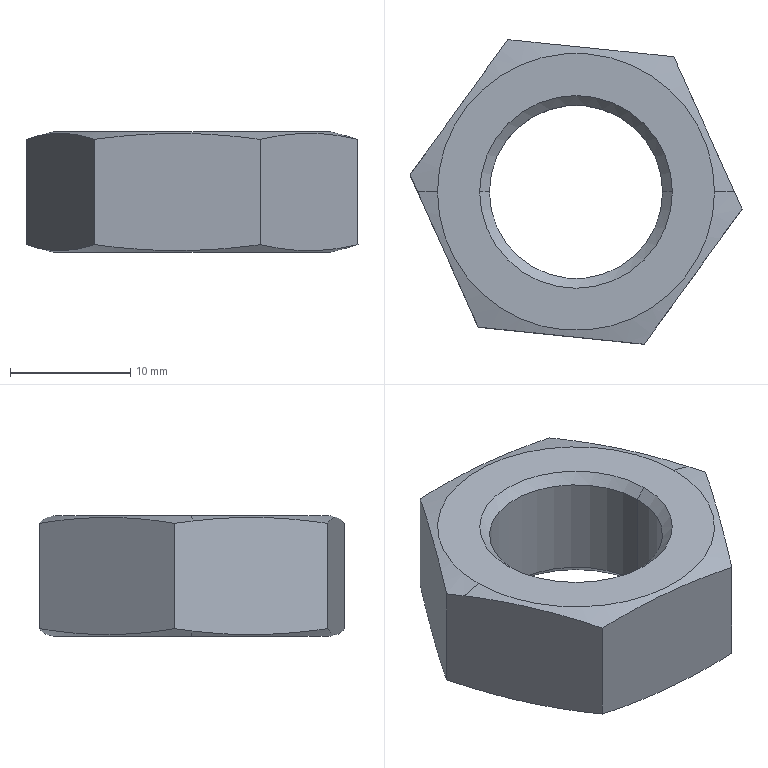Part | SolidWorks | features BaseBody 1 | 1 solid | 18 faces | box 27.567 x 25.293 x 10 mm | volume 3303 mm3 | cone 8 | plane 8 | cylinder 2 | commonest cylinder face diameters 14.376 x2
STEP:
#1=CARTESIAN_POINT('',(223.5,0.,-23.475));
#2=VERTEX_POINT('',#1);
#3=CARTESIAN_POINT('',(246.5,0.,-23.475));
#4=VERTEX_POINT('',#3);
#5=CARTESIAN_POINT('',(235.,0.,-23.475));
#6=DIRECTION('',(0.,0.,-1.));
#7=DIRECTION('',(1.,0.,0.));
#8=AXIS2_PLACEMENT_3D('',#5,#6,#7);
#9=CIRCLE('',#8,11.5);
#10=EDGE_CURVE('',#2,#4,#9,.T.);
#11=ORIENTED_EDGE('',*,*,#10,.F.);
#12=CARTESIAN_POINT('',(221.852,0.,-23.033));
#13=VERTEX_POINT('',#12);
#14=CARTESIAN_POINT('',(221.129,0.,-22.839));
#15=DIRECTION('',(-0.9659,0.,0.2588));
#16=VECTOR('',#15,1000.);
#17=LINE('',#14,#16);
#18=EDGE_CURVE('',#2,#13,#17,.T.);
#19=ORIENTED_EDGE('',*,*,#18,.T.);
#20=CARTESIAN_POINT('',(221.216,1.419,-22.843));
#21=VERTEX_POINT('',#20);
#22=CARTESIAN_POINT('',(221.852,0.,-23.033));
#23=CARTESIAN_POINT('',(221.64,0.4732,-22.976));
#24=CARTESIAN_POINT('',(221.428,0.9463,-22.913));
#25=CARTESIAN_POINT('',(221.216,1.419,-22.843));
#26=B_SPLINE_CURVE_WITH_KNOTS('',3,(#22,#23,#24,#25),.UNSPECIFIED.,.F.,.F.,(4,4),(0.0123,0.01386),.UNSPECIFIED.);
#27=EDGE_CURVE('',#13,#21,#26,.T.);
#28=ORIENTED_EDGE('',*,*,#27,.T.);
#29=CARTESIAN_POINT('',(229.338,12.647,-22.843));
#30=VERTEX_POINT('',#29);
#31=CARTESIAN_POINT('',(221.216,1.419,-22.843));
#32=CARTESIAN_POINT('',(221.893,2.355,-22.998));
#33=CARTESIAN_POINT('',(222.57,3.291,-23.124));
#34=CARTESIAN_POINT('',(223.924,5.162,-23.295));
#35=CARTESIAN_POINT('',(225.277,7.033,-23.386));
#36=CARTESIAN_POINT('',(226.631,8.904,-23.295));
#37=CARTESIAN_POINT('',(227.984,10.775,-23.124));
#38=CARTESIAN_POINT('',(228.661,11.711,-22.998));
#39=CARTESIAN_POINT('',(229.338,12.647,-22.843));
#40=B_SPLINE_CURVE_WITH_KNOTS('',3,(#31,#32,#33,#34,#35,#36,#37,#38,#39),.UNSPECIFIED.,.F.,.F.,(4,2,1,2,4),(0.,0.003464,0.006928,0.01039,0.01386),.UNSPECIFIED.);
#41=EDGE_CURVE('',#21,#30,#40,.T.);
#42=ORIENTED_EDGE('',*,*,#41,.T.);
#43=CARTESIAN_POINT('',(243.121,11.227,-22.843));
#44=VERTEX_POINT('',#43);
#45=CARTESIAN_POINT('',(229.338,12.647,-22.843));
#46=CARTESIAN_POINT('',(230.481,12.529,-22.997));
#47=CARTESIAN_POINT('',(231.627,12.411,-23.123));
#48=CARTESIAN_POINT('',(233.924,12.174,-23.295));
#49=CARTESIAN_POINT('',(235.075,12.056,-23.341));
#50=CARTESIAN_POINT('',(237.384,11.818,-23.341));
#51=CARTESIAN_POINT('',(238.535,11.699,-23.295));
#52=CARTESIAN_POINT('',(240.832,11.463,-23.123));
#53=CARTESIAN_POINT('',(241.978,11.345,-22.997));
#54=CARTESIAN_POINT('',(243.121,11.227,-22.843));
#55=B_SPLINE_CURVE_WITH_KNOTS('',3,(#45,#46,#47,#48,#49,#50,#51,#52,#53,#54),.UNSPECIFIED.,.F.,.F.,(4,2,2,2,4),(-0.006946,-0.003473,0.,0.003473,0.006946),.UNSPECIFIED.);
#56=EDGE_CURVE('',#30,#44,#55,.T.);
#57=ORIENTED_EDGE('',*,*,#56,.T.);
#58=CARTESIAN_POINT('',(248.148,0.,-23.033));
#59=VERTEX_POINT('',#58);
#60=CARTESIAN_POINT('',(243.121,11.227,-22.843));
#61=CARTESIAN_POINT('',(243.959,9.356,-23.118));
#62=CARTESIAN_POINT('',(244.797,7.485,-23.298));
#63=CARTESIAN_POINT('',(246.053,4.678,-23.352));
#64=CARTESIAN_POINT('',(246.472,3.742,-23.334));
#65=CARTESIAN_POINT('',(247.31,1.871,-23.231));
#66=CARTESIAN_POINT('',(247.729,0.9356,-23.145));
#67=CARTESIAN_POINT('',(248.148,0.,-23.033));
#68=B_SPLINE_CURVE_WITH_KNOTS('',3,(#60,#61,#62,#63,#64,#65,#66,#67),.UNSPECIFIED.,.F.,.F.,(4,2,2,4),(0.,0.006151,0.009226,0.0123),.UNSPECIFIED.);
#69=EDGE_CURVE('',#44,#59,#68,.T.);
#70=ORIENTED_EDGE('',*,*,#69,.T.);
#71=CARTESIAN_POINT('',(248.871,0.,-22.839));
#72=DIRECTION('',(0.9659,0.,0.2588));
#73=VECTOR('',#72,1000.);
#74=LINE('',#71,#73);
#75=EDGE_CURVE('',#4,#59,#74,.T.);
#76=ORIENTED_EDGE('',*,*,#75,.F.);
#77=EDGE_LOOP('',(#11,#19,#28,#42,#57,#70,#76));
#78=FACE_OUTER_BOUND('',#77,.T.);
#79=CARTESIAN_POINT('',(235.,0.,-22.839));
#80=DIRECTION('',(0.,0.,1.));
#81=DIRECTION('',(1.,0.,0.));
#82=AXIS2_PLACEMENT_3D('',#79,#80,#81);
#83=CONICAL_SURFACE('',#82,13.871,1.309);
#84=ADVANCED_FACE('',(#78),#83,.T.);
#85=CARTESIAN_POINT('',(242.188,0.,-22.663));
#86=VERTEX_POINT('',#85);
#87=CARTESIAN_POINT('',(227.812,0.,-22.663));
#88=VERTEX_POINT('',#87);
#89=CARTESIAN_POINT('',(235.,0.,-22.663));
#90=DIRECTION('',(0.,0.,-1.));
#91=DIRECTION('',(0.1024,0.9947,0.));
#92=AXIS2_PLACEMENT_3D('',#89,#90,#91);
#93=CIRCLE('',#92,7.188);
#94=EDGE_CURVE('',#86,#88,#93,.T.);
#95=ORIENTED_EDGE('',*,*,#94,.F.);
#96=CARTESIAN_POINT('',(243.,0.,-23.475));
#97=VERTEX_POINT('',#96);
#98=CARTESIAN_POINT('',(243.,0.,-23.475));
#99=DIRECTION('',(0.7071,0.,-0.7071));
#100=VECTOR('',#99,1000.);
#101=LINE('',#98,#100);
#102=EDGE_CURVE('',#86,#97,#101,.T.);
#103=ORIENTED_EDGE('',*,*,#102,.T.);
#104=CARTESIAN_POINT('',(227.,0.,-23.475));
#105=VERTEX_POINT('',#104);
#106=CARTESIAN_POINT('',(235.,0.,-23.475));
#107=DIRECTION('',(0.,0.,1.));
#108=DIRECTION('',(-1.,0.,0.));
#109=AXIS2_PLACEMENT_3D('',#106,#107,#108);
#110=CIRCLE('',#109,8.);
#111=EDGE_CURVE('',#105,#97,#110,.T.);
#112=ORIENTED_EDGE('',*,*,#111,.F.);
#113=CARTESIAN_POINT('',(227.,0.,-23.475));
#114=DIRECTION('',(-0.7071,0.,-0.7071));
#115=VECTOR('',#114,1000.);
#116=LINE('',#113,#115);
#117=EDGE_CURVE('',#88,#105,#116,.T.);
#118=ORIENTED_EDGE('',*,*,#117,.F.);
#119=EDGE_LOOP('',(#95,#103,#112,#118));
#120=FACE_OUTER_BOUND('',#119,.T.);
#121=CARTESIAN_POINT('',(235.,0.,-23.475));
#122=DIRECTION('',(0.,0.,-1.));
#123=DIRECTION('',(-1.,0.,0.));
#124=AXIS2_PLACEMENT_3D('',#121,#122,#123);
#125=CONICAL_SURFACE('',#124,8.,0.7854);
#126=ADVANCED_FACE('',(#120),#125,.F.);
#127=CARTESIAN_POINT('',(242.188,0.,-14.287));
#128=VERTEX_POINT('',#127);
#129=CARTESIAN_POINT('',(227.812,0.,-14.287));
#130=VERTEX_POINT('',#129);
#131=CARTESIAN_POINT('',(235.,0.,-14.287));
#132=DIRECTION('',(0.,0.,-1.));
#133=DIRECTION('',(-1.,0.,0.));
#134=AXIS2_PLACEMENT_3D('',#131,#132,#133);
#135=CIRCLE('',#134,7.188);
#136=EDGE_CURVE('',#128,#130,#135,.T.);
#137=ORIENTED_EDGE('',*,*,#136,.F.);
#138=CARTESIAN_POINT('',(242.188,0.,-18.475));
#139=DIRECTION('',(0.,0.,-1.));
#140=VECTOR('',#139,1000.);
#141=LINE('',#138,#140);
#142=EDGE_CURVE('',#128,#86,#141,.T.);
#143=ORIENTED_EDGE('',*,*,#142,.T.);
#144=ORIENTED_EDGE('',*,*,#94,.T.);
#145=CARTESIAN_POINT('',(227.812,0.,-18.475));
#146=DIRECTION('',(0.,0.,-1.));
#147=VECTOR('',#146,1000.);
#148=LINE('',#145,#147);
#149=EDGE_CURVE('',#130,#88,#148,.T.);
#150=ORIENTED_EDGE('',*,*,#149,.F.);
#151=EDGE_LOOP('',(#137,#143,#144,#150));
#152=FACE_OUTER_BOUND('',#151,.T.);
#153=CARTESIAN_POINT('',(235.,0.,-18.475));
#154=DIRECTION('',(0.,0.,-1.));
#155=DIRECTION('',(-1.,0.,0.));
#156=AXIS2_PLACEMENT_3D('',#153,#154,#155);
#157=CYLINDRICAL_SURFACE('',#156,7.188);
#158=ADVANCED_FACE('',(#152),#157,.F.);
#159=CARTESIAN_POINT('',(223.5,0.,-13.475));
#160=VERTEX_POINT('',#159);
#161=CARTESIAN_POINT('',(246.5,0.,-13.475));
#162=VERTEX_POINT('',#161);
#163=CARTESIAN_POINT('',(235.,0.,-13.475));
#164=DIRECTION('',(0.,0.,-1.));
#165=DIRECTION('',(-1.,0.,0.));
#166=AXIS2_PLACEMENT_3D('',#163,#164,#165);
#167=CIRCLE('',#166,11.5);
#168=EDGE_CURVE('',#160,#162,#167,.T.);
#169=ORIENTED_EDGE('',*,*,#168,.T.);
#170=CARTESIAN_POINT('',(248.148,0.,-13.916));
#171=VERTEX_POINT('',#170);
#172=CARTESIAN_POINT('',(248.871,0.,-14.11));
#173=DIRECTION('',(0.9659,0.,-0.2588));
#174=VECTOR('',#173,1000.);
#175=LINE('',#172,#174);
#176=EDGE_CURVE('',#162,#171,#175,.T.);
#177=ORIENTED_EDGE('',*,*,#176,.T.);
#178=CARTESIAN_POINT('',(243.121,11.227,-14.106));
#179=VERTEX_POINT('',#178);
#180=CARTESIAN_POINT('',(248.148,0.,-13.916));
#181=CARTESIAN_POINT('',(247.729,0.9356,-13.804));
#182=CARTESIAN_POINT('',(247.31,1.871,-13.719));
#183=CARTESIAN_POINT('',(246.472,3.742,-13.615));
#184=CARTESIAN_POINT('',(246.053,4.678,-13.598));
#185=CARTESIAN_POINT('',(244.797,7.485,-13.651));
#186=CARTESIAN_POINT('',(243.959,9.356,-13.831));
#187=CARTESIAN_POINT('',(243.121,11.227,-14.106));
#188=B_SPLINE_CURVE_WITH_KNOTS('',3,(#180,#181,#182,#183,#184,#185,#186,#187),.UNSPECIFIED.,.F.,.F.,(4,2,2,4),(0.001555,0.004631,0.007706,0.01386),.UNSPECIFIED.);
#189=EDGE_CURVE('',#171,#179,#188,.T.);
#190=ORIENTED_EDGE('',*,*,#189,.T.);
#191=CARTESIAN_POINT('',(229.338,12.647,-14.106));
#192=VERTEX_POINT('',#191);
#193=CARTESIAN_POINT('',(243.121,11.227,-14.106));
#194=CARTESIAN_POINT('',(241.978,11.345,-13.952));
#195=CARTESIAN_POINT('',(240.832,11.463,-13.826));
#196=CARTESIAN_POINT('',(238.535,11.699,-13.655));
#197=CARTESIAN_POINT('',(237.384,11.818,-13.609));
#198=CARTESIAN_POINT('',(235.075,12.056,-13.609));
#199=CARTESIAN_POINT('',(233.924,12.174,-13.655));
#200=CARTESIAN_POINT('',(231.627,12.411,-13.826));
#201=CARTESIAN_POINT('',(230.481,12.529,-13.952));
#202=CARTESIAN_POINT('',(229.338,12.647,-14.106));
#203=B_SPLINE_CURVE_WITH_KNOTS('',3,(#193,#194,#195,#196,#197,#198,#199,#200,#201,#202),.UNSPECIFIED.,.F.,.F.,(4,2,2,2,4),(-0.006946,-0.003473,0.,0.003473,0.006946),.UNSPECIFIED.);
#204=EDGE_CURVE('',#179,#192,#203,.T.);
#205=ORIENTED_EDGE('',*,*,#204,.T.);
#206=CARTESIAN_POINT('',(221.216,1.419,-14.106));
#207=VERTEX_POINT('',#206);
#208=CARTESIAN_POINT('',(229.338,12.647,-14.106));
#209=CARTESIAN_POINT('',(228.661,11.711,-13.951));
#210=CARTESIAN_POINT('',(227.984,10.775,-13.826));
#211=CARTESIAN_POINT('',(226.631,8.904,-13.654));
#212=CARTESIAN_POINT('',(225.277,7.033,-13.563));
#213=CARTESIAN_POINT('',(223.924,5.162,-13.654));
#214=CARTESIAN_POINT('',(222.57,3.291,-13.826));
#215=CARTESIAN_POINT('',(221.893,2.355,-13.951));
#216=CARTESIAN_POINT('',(221.216,1.419,-14.106));
#217=B_SPLINE_CURVE_WITH_KNOTS('',3,(#208,#209,#210,#211,#212,#213,#214,#215,#216),.UNSPECIFIED.,.F.,.F.,(4,2,1,2,4),(0.,0.003464,0.006928,0.01039,0.01386),.UNSPECIFIED.);
#218=EDGE_CURVE('',#192,#207,#217,.T.);
#219=ORIENTED_EDGE('',*,*,#218,.T.);
#220=CARTESIAN_POINT('',(221.852,0.,-13.916));
#221=VERTEX_POINT('',#220);
#222=CARTESIAN_POINT('',(221.216,1.419,-14.106));
#223=CARTESIAN_POINT('',(221.428,0.9463,-14.037));
#224=CARTESIAN_POINT('',(221.64,0.4732,-13.973));
#225=CARTESIAN_POINT('',(221.852,0.,-13.916));
#226=B_SPLINE_CURVE_WITH_KNOTS('',3,(#222,#223,#224,#225),.UNSPECIFIED.,.F.,.F.,(4,4),(0.,0.001555),.UNSPECIFIED.);
#227=EDGE_CURVE('',#207,#221,#226,.T.);
#228=ORIENTED_EDGE('',*,*,#227,.T.);
#229=CARTESIAN_POINT('',(221.129,0.,-14.11));
#230=DIRECTION('',(-0.9659,0.,-0.2588));
#231=VECTOR('',#230,1000.);
#232=LINE('',#229,#231);
#233=EDGE_CURVE('',#160,#221,#232,.T.);
#234=ORIENTED_EDGE('',*,*,#233,.F.);
#235=EDGE_LOOP('',(#169,#177,#190,#205,#219,#228,#234));
#236=FACE_OUTER_BOUND('',#235,.T.);
#237=CARTESIAN_POINT('',(235.,0.,-14.11));
#238=DIRECTION('',(0.,0.,-1.));
#239=DIRECTION('',(-1.,0.,0.));
#240=AXIS2_PLACEMENT_3D('',#237,#238,#239);
#241=CONICAL_SURFACE('',#240,13.871,1.309);
#242=ADVANCED_FACE('',(#236),#241,.T.);
#243=ORIENTED_EDGE('',*,*,#136,.T.);
#244=CARTESIAN_POINT('',(227.,0.,-13.475));
#245=VERTEX_POINT('',#244);
#246=CARTESIAN_POINT('',(227.,0.,-13.475));
#247=DIRECTION('',(-0.7071,0.,0.7071));
#248=VECTOR('',#247,1000.);
#249=LINE('',#246,#248);
#250=EDGE_CURVE('',#130,#245,#249,.T.);
#251=ORIENTED_EDGE('',*,*,#250,.T.);
#252=CARTESIAN_POINT('',(243.,0.,-13.475));
#253=VERTEX_POINT('',#252);
#254=CARTESIAN_POINT('',(235.,0.,-13.475));
#255=DIRECTION('',(0.,0.,-1.));
#256=DIRECTION('',(1.,0.,0.));
#257=AXIS2_PLACEMENT_3D('',#254,#255,#256);
#258=CIRCLE('',#257,8.);
#259=EDGE_CURVE('',#253,#245,#258,.T.);
#260=ORIENTED_EDGE('',*,*,#259,.F.);
#261=CARTESIAN_POINT('',(243.,0.,-13.475));
#262=DIRECTION('',(0.7071,0.,0.7071));
#263=VECTOR('',#262,1000.);
#264=LINE('',#261,#263);
#265=EDGE_CURVE('',#128,#253,#264,.T.);
#266=ORIENTED_EDGE('',*,*,#265,.F.);
#267=EDGE_LOOP('',(#243,#251,#260,#266));
#268=FACE_OUTER_BOUND('',#267,.T.);
#269=CARTESIAN_POINT('',(235.,0.,-13.475));
#270=DIRECTION('',(0.,0.,1.));
#271=DIRECTION('',(1.,0.,0.));
#272=AXIS2_PLACEMENT_3D('',#269,#270,#271);
#273=CONICAL_SURFACE('',#272,8.,0.7854);
#274=ADVANCED_FACE('',(#268),#273,.F.);
#275=CARTESIAN_POINT('',(235.,0.,-23.475));
#276=DIRECTION('',(0.,0.,-1.));
#277=DIRECTION('',(1.,0.,0.));
#278=AXIS2_PLACEMENT_3D('',#275,#276,#277);
#279=CIRCLE('',#278,11.5);
#280=EDGE_CURVE('',#4,#2,#279,.T.);
#281=ORIENTED_EDGE('',*,*,#280,.T.);
#282=ORIENTED_EDGE('',*,*,#10,.T.);
#283=EDGE_LOOP('',(#281,#282));
#284=FACE_OUTER_BOUND('',#283,.T.);
#285=ORIENTED_EDGE('',*,*,#111,.T.);
#286=CARTESIAN_POINT('',(235.,0.,-23.475));
#287=DIRECTION('',(0.,0.,1.));
#288=DIRECTION('',(-1.,0.,0.));
#289=AXIS2_PLACEMENT_3D('',#286,#287,#288);
#290=CIRCLE('',#289,8.);
#291=EDGE_CURVE('',#97,#105,#290,.T.);
#292=ORIENTED_EDGE('',*,*,#291,.T.);
#293=EDGE_LOOP('',(#285,#292));
#294=FACE_BOUND('',#293,.T.);
#295=CARTESIAN_POINT('',(225.301,0.9988,-23.475));
#296=DIRECTION('',(0.,0.,-1.));
#297=DIRECTION('',(-1.,0.,0.));
#298=AXIS2_PLACEMENT_3D('',#295,#296,#297);
#299=PLANE('',#298);
#300=ADVANCED_FACE('',(#284,#294),#299,.T.);
#301=ORIENTED_EDGE('',*,*,#18,.F.);
#302=ORIENTED_EDGE('',*,*,#280,.F.);
#303=ORIENTED_EDGE('',*,*,#75,.T.);
#304=CARTESIAN_POINT('',(248.784,-1.419,-22.843));
#305=VERTEX_POINT('',#304);
#306=CARTESIAN_POINT('',(248.148,0.,-23.033));
#307=CARTESIAN_POINT('',(248.36,-0.4732,-22.976));
#308=CARTESIAN_POINT('',(248.572,-0.9463,-22.913));
#309=CARTESIAN_POINT('',(248.784,-1.419,-22.843));
#310=B_SPLINE_CURVE_WITH_KNOTS('',3,(#306,#307,#308,#309),.UNSPECIFIED.,.F.,.F.,(4,4),(0.0123,0.01386),.UNSPECIFIED.);
#311=EDGE_CURVE('',#59,#305,#310,.T.);
#312=ORIENTED_EDGE('',*,*,#311,.T.);
#313=CARTESIAN_POINT('',(240.662,-12.647,-22.843));
#314=VERTEX_POINT('',#313);
#315=CARTESIAN_POINT('',(248.784,-1.419,-22.843));
#316=CARTESIAN_POINT('',(248.107,-2.355,-22.998));
#317=CARTESIAN_POINT('',(247.43,-3.291,-23.124));
#318=CARTESIAN_POINT('',(246.076,-5.162,-23.295));
#319=CARTESIAN_POINT('',(244.723,-7.033,-23.386));
#320=CARTESIAN_POINT('',(243.369,-8.904,-23.295));
#321=CARTESIAN_POINT('',(242.016,-10.775,-23.124));
#322=CARTESIAN_POINT('',(241.339,-11.711,-22.998));
#323=CARTESIAN_POINT('',(240.662,-12.647,-22.843));
#324=B_SPLINE_CURVE_WITH_KNOTS('',3,(#315,#316,#317,#318,#319,#320,#321,#322,#323),.UNSPECIFIED.,.F.,.F.,(4,2,1,2,4),(0.,0.003464,0.006928,0.01039,0.01386),.UNSPECIFIED.);
#325=EDGE_CURVE('',#305,#314,#324,.T.);
#326=ORIENTED_EDGE('',*,*,#325,.T.);
#327=CARTESIAN_POINT('',(226.879,-11.227,-22.843));
#328=VERTEX_POINT('',#327);
#329=CARTESIAN_POINT('',(240.662,-12.647,-22.843));
#330=CARTESIAN_POINT('',(239.519,-12.529,-22.997));
#331=CARTESIAN_POINT('',(238.373,-12.411,-23.123));
#332=CARTESIAN_POINT('',(236.076,-12.174,-23.295));
#333=CARTESIAN_POINT('',(234.925,-12.056,-23.341));
#334=CARTESIAN_POINT('',(232.616,-11.818,-23.341));
#335=CARTESIAN_POINT('',(231.465,-11.699,-23.295));
#336=CARTESIAN_POINT('',(229.168,-11.463,-23.123));
#337=CARTESIAN_POINT('',(228.022,-11.345,-22.997));
#338=CARTESIAN_POINT('',(226.879,-11.227,-22.843));
#339=B_SPLINE_CURVE_WITH_KNOTS('',3,(#329,#330,#331,#332,#333,#334,#335,#336,#337,#338),.UNSPECIFIED.,.F.,.F.,(4,2,2,2,4),(-0.006946,-0.003473,0.,0.003473,0.006946),.UNSPECIFIED.);
#340=EDGE_CURVE('',#314,#328,#339,.T.);
#341=ORIENTED_EDGE('',*,*,#340,.T.);
#342=CARTESIAN_POINT('',(226.879,-11.227,-22.843));
#343=CARTESIAN_POINT('',(226.041,-9.356,-23.118));
#344=CARTESIAN_POINT('',(225.203,-7.485,-23.298));
#345=CARTESIAN_POINT('',(223.947,-4.678,-23.352));
#346=CARTESIAN_POINT('',(223.528,-3.742,-23.334));
#347=CARTESIAN_POINT('',(222.69,-1.871,-23.231));
#348=CARTESIAN_POINT('',(222.271,-0.9356,-23.145));
#349=CARTESIAN_POINT('',(221.852,0.,-23.033));
#350=B_SPLINE_CURVE_WITH_KNOTS('',3,(#342,#343,#344,#345,#346,#347,#348,#349),.UNSPECIFIED.,.F.,.F.,(4,2,2,4),(0.,0.006151,0.009226,0.0123),.UNSPECIFIED.);
#351=EDGE_CURVE('',#328,#13,#350,.T.);
#352=ORIENTED_EDGE('',*,*,#351,.T.);
#353=EDGE_LOOP('',(#301,#302,#303,#312,#326,#341,#352));
#354=FACE_OUTER_BOUND('',#353,.T.);
#355=CARTESIAN_POINT('',(235.,0.,-22.839));
#356=DIRECTION('',(0.,0.,1.));
#357=DIRECTION('',(1.,0.,0.));
#358=AXIS2_PLACEMENT_3D('',#355,#356,#357);
#359=CONICAL_SURFACE('',#358,13.871,1.309);
#360=ADVANCED_FACE('',(#354),#359,.T.);
#361=ORIENTED_EDGE('',*,*,#102,.F.);
#362=CARTESIAN_POINT('',(235.,0.,-22.663));
#363=DIRECTION('',(0.,0.,-1.));
#364=DIRECTION('',(0.1024,0.9947,0.));
#365=AXIS2_PLACEMENT_3D('',#362,#363,#364);
#366=CIRCLE('',#365,7.188);
#367=EDGE_CURVE('',#88,#86,#366,.T.);
#368=ORIENTED_EDGE('',*,*,#367,.F.);
#369=ORIENTED_EDGE('',*,*,#117,.T.);
#370=ORIENTED_EDGE('',*,*,#291,.F.);
#371=EDGE_LOOP('',(#361,#368,#369,#370));
#372=FACE_OUTER_BOUND('',#371,.T.);
#373=CARTESIAN_POINT('',(235.,0.,-23.475));
#374=DIRECTION('',(0.,0.,-1.));
#375=DIRECTION('',(-1.,0.,0.));
#376=AXIS2_PLACEMENT_3D('',#373,#374,#375);
#377=CONICAL_SURFACE('',#376,8.,0.7854);
#378=ADVANCED_FACE('',(#372),#377,.F.);
#379=CARTESIAN_POINT('',(248.784,-1.419,-14.106));
#380=VERTEX_POINT('',#379);
#381=CARTESIAN_POINT('',(248.784,-1.419,-14.106));
#382=CARTESIAN_POINT('',(248.572,-0.9463,-14.037));
#383=CARTESIAN_POINT('',(248.36,-0.4732,-13.973));
#384=CARTESIAN_POINT('',(248.148,0.,-13.916));
#385=B_SPLINE_CURVE_WITH_KNOTS('',3,(#381,#382,#383,#384),.UNSPECIFIED.,.F.,.F.,(4,4),(0.,0.001555),.UNSPECIFIED.);
#386=EDGE_CURVE('',#380,#171,#385,.T.);
#387=ORIENTED_EDGE('',*,*,#386,.F.);
#388=CARTESIAN_POINT('',(248.784,-1.419,-23.475));
#389=DIRECTION('',(0.,0.,1.));
#390=VECTOR('',#389,1000.);
#391=LINE('',#388,#390);
#392=EDGE_CURVE('',#305,#380,#391,.T.);
#393=ORIENTED_EDGE('',*,*,#392,.F.);
#394=ORIENTED_EDGE('',*,*,#311,.F.);
#395=ORIENTED_EDGE('',*,*,#69,.F.);
#396=CARTESIAN_POINT('',(243.121,11.227,-23.475));
#397=DIRECTION('',(0.,0.,-1.));
#398=VECTOR('',#397,1000.);
#399=LINE('',#396,#398);
#400=EDGE_CURVE('',#179,#44,#399,.T.);
#401=ORIENTED_EDGE('',*,*,#400,.F.);
#402=ORIENTED_EDGE('',*,*,#189,.F.);
#403=EDGE_LOOP('',(#387,#393,#394,#395,#401,#402));
#404=FACE_OUTER_BOUND('',#403,.T.);
#405=CARTESIAN_POINT('',(248.784,-1.419,-23.475));
#406=DIRECTION('',(-0.9127,-0.4087,0.));
#407=DIRECTION('',(0.4087,-0.9127,0.));
#408=AXIS2_PLACEMENT_3D('',#405,#406,#407);
#409=PLANE('',#408);
#410=ADVANCED_FACE('',(#404),#409,.F.);
#411=ORIENTED_EDGE('',*,*,#204,.F.);
#412=ORIENTED_EDGE('',*,*,#400,.T.);
#413=ORIENTED_EDGE('',*,*,#56,.F.);
#414=CARTESIAN_POINT('',(229.338,12.647,-23.475));
#415=DIRECTION('',(0.,0.,-1.));
#416=VECTOR('',#415,1000.);
#417=LINE('',#414,#416);
#418=EDGE_CURVE('',#192,#30,#417,.T.);
#419=ORIENTED_EDGE('',*,*,#418,.F.);
#420=EDGE_LOOP('',(#411,#412,#413,#419));
#421=FACE_OUTER_BOUND('',#420,.T.);
#422=CARTESIAN_POINT('',(243.121,11.227,-23.475));
#423=DIRECTION('',(-0.1024,-0.9947,0.));
#424=DIRECTION('',(0.9947,-0.1024,0.));
#425=AXIS2_PLACEMENT_3D('',#422,#423,#424);
#426=PLANE('',#425);
#427=ADVANCED_FACE('',(#421),#426,.F.);
#428=ORIENTED_EDGE('',*,*,#218,.F.);
#429=ORIENTED_EDGE('',*,*,#418,.T.);
#430=ORIENTED_EDGE('',*,*,#41,.F.);
#431=CARTESIAN_POINT('',(221.216,1.419,-23.475));
#432=DIRECTION('',(0.,0.,-1.));
#433=VECTOR('',#432,1000.);
#434=LINE('',#431,#433);
#435=EDGE_CURVE('',#207,#21,#434,.T.);
#436=ORIENTED_EDGE('',*,*,#435,.F.);
#437=EDGE_LOOP('',(#428,#429,#430,#436));
#438=FACE_OUTER_BOUND('',#437,.T.);
#439=CARTESIAN_POINT('',(229.338,12.647,-23.475));
#440=DIRECTION('',(0.8102,-0.5861,0.));
#441=DIRECTION('',(0.5861,0.8102,0.));
#442=AXIS2_PLACEMENT_3D('',#439,#440,#441);
#443=PLANE('',#442);
#444=ADVANCED_FACE('',(#438),#443,.F.);
#445=ORIENTED_EDGE('',*,*,#227,.F.);
#446=ORIENTED_EDGE('',*,*,#435,.T.);
#447=ORIENTED_EDGE('',*,*,#27,.F.);
#448=ORIENTED_EDGE('',*,*,#351,.F.);
#449=CARTESIAN_POINT('',(226.879,-11.227,-14.106));
#450=VERTEX_POINT('',#449);
#451=CARTESIAN_POINT('',(226.879,-11.227,-23.475));
#452=DIRECTION('',(0.,0.,-1.));
#453=VECTOR('',#452,1000.);
#454=LINE('',#451,#453);
#455=EDGE_CURVE('',#450,#328,#454,.T.);
#456=ORIENTED_EDGE('',*,*,#455,.F.);
#457=CARTESIAN_POINT('',(221.852,0.,-13.916));
#458=CARTESIAN_POINT('',(222.271,-0.9356,-13.804));
#459=CARTESIAN_POINT('',(222.69,-1.871,-13.719));
#460=CARTESIAN_POINT('',(223.528,-3.742,-13.615));
#461=CARTESIAN_POINT('',(223.947,-4.678,-13.598));
#462=CARTESIAN_POINT('',(225.203,-7.485,-13.651));
#463=CARTESIAN_POINT('',(226.041,-9.356,-13.831));
#464=CARTESIAN_POINT('',(226.879,-11.227,-14.106));
#465=B_SPLINE_CURVE_WITH_KNOTS('',3,(#457,#458,#459,#460,#461,#462,#463,#464),.UNSPECIFIED.,.F.,.F.,(4,2,2,4),(0.001555,0.004631,0.007706,0.01386),.UNSPECIFIED.);
#466=EDGE_CURVE('',#221,#450,#465,.T.);
#467=ORIENTED_EDGE('',*,*,#466,.F.);
#468=EDGE_LOOP('',(#445,#446,#447,#448,#456,#467));
#469=FACE_OUTER_BOUND('',#468,.T.);
#470=CARTESIAN_POINT('',(221.216,1.419,-23.475));
#471=DIRECTION('',(0.9127,0.4087,0.));
#472=DIRECTION('',(-0.4087,0.9127,0.));
#473=AXIS2_PLACEMENT_3D('',#470,#471,#472);
#474=PLANE('',#473);
#475=ADVANCED_FACE('',(#469),#474,.F.);
#476=CARTESIAN_POINT('',(240.662,-12.647,-14.106));
#477=VERTEX_POINT('',#476);
#478=CARTESIAN_POINT('',(226.879,-11.227,-14.106));
#479=CARTESIAN_POINT('',(228.022,-11.345,-13.952));
#480=CARTESIAN_POINT('',(229.168,-11.463,-13.826));
#481=CARTESIAN_POINT('',(231.465,-11.699,-13.655));
#482=CARTESIAN_POINT('',(232.616,-11.818,-13.609));
#483=CARTESIAN_POINT('',(234.925,-12.056,-13.609));
#484=CARTESIAN_POINT('',(236.076,-12.174,-13.655));
#485=CARTESIAN_POINT('',(238.373,-12.411,-13.826));
#486=CARTESIAN_POINT('',(239.519,-12.529,-13.952));
#487=CARTESIAN_POINT('',(240.662,-12.647,-14.106));
#488=B_SPLINE_CURVE_WITH_KNOTS('',3,(#478,#479,#480,#481,#482,#483,#484,#485,#486,#487),.UNSPECIFIED.,.F.,.F.,(4,2,2,2,4),(-0.006946,-0.003473,0.,0.003473,0.006946),.UNSPECIFIED.);
#489=EDGE_CURVE('',#450,#477,#488,.T.);
#490=ORIENTED_EDGE('',*,*,#489,.F.);
#491=ORIENTED_EDGE('',*,*,#455,.T.);
#492=ORIENTED_EDGE('',*,*,#340,.F.);
#493=CARTESIAN_POINT('',(240.662,-12.647,-23.475));
#494=DIRECTION('',(0.,0.,-1.));
#495=VECTOR('',#494,1000.);
#496=LINE('',#493,#495);
#497=EDGE_CURVE('',#477,#314,#496,.T.);
#498=ORIENTED_EDGE('',*,*,#497,.F.);
#499=EDGE_LOOP('',(#490,#491,#492,#498));
#500=FACE_OUTER_BOUND('',#499,.T.);
#501=CARTESIAN_POINT('',(226.879,-11.227,-23.475));
#502=DIRECTION('',(0.1024,0.9947,0.));
#503=DIRECTION('',(-0.9947,0.1024,0.));
#504=AXIS2_PLACEMENT_3D('',#501,#502,#503);
#505=PLANE('',#504);
#506=ADVANCED_FACE('',(#500),#505,.F.);
#507=CARTESIAN_POINT('',(240.662,-12.647,-14.106));
#508=CARTESIAN_POINT('',(241.339,-11.711,-13.951));
#509=CARTESIAN_POINT('',(242.016,-10.775,-13.826));
#510=CARTESIAN_POINT('',(243.369,-8.904,-13.654));
#511=CARTESIAN_POINT('',(244.723,-7.033,-13.563));
#512=CARTESIAN_POINT('',(246.076,-5.162,-13.654));
#513=CARTESIAN_POINT('',(247.43,-3.291,-13.826));
#514=CARTESIAN_POINT('',(248.107,-2.355,-13.951));
#515=CARTESIAN_POINT('',(248.784,-1.419,-14.106));
#516=B_SPLINE_CURVE_WITH_KNOTS('',3,(#507,#508,#509,#510,#511,#512,#513,#514,#515),.UNSPECIFIED.,.F.,.F.,(4,2,1,2,4),(0.,0.003464,0.006928,0.01039,0.01386),.UNSPECIFIED.);
#517=EDGE_CURVE('',#477,#380,#516,.T.);
#518=ORIENTED_EDGE('',*,*,#517,.F.);
#519=ORIENTED_EDGE('',*,*,#497,.T.);
#520=ORIENTED_EDGE('',*,*,#325,.F.);
#521=ORIENTED_EDGE('',*,*,#392,.T.);
#522=EDGE_LOOP('',(#518,#519,#520,#521));
#523=FACE_OUTER_BOUND('',#522,.T.);
#524=CARTESIAN_POINT('',(240.662,-12.647,-23.475));
#525=DIRECTION('',(-0.8102,0.5861,0.));
#526=DIRECTION('',(-0.5861,-0.8102,0.));
#527=AXIS2_PLACEMENT_3D('',#524,#525,#526);
#528=PLANE('',#527);
#529=ADVANCED_FACE('',(#523),#528,.F.);
#530=ORIENTED_EDGE('',*,*,#142,.F.);
#531=CARTESIAN_POINT('',(235.,0.,-14.287));
#532=DIRECTION('',(0.,0.,-1.));
#533=DIRECTION('',(-1.,0.,0.));
#534=AXIS2_PLACEMENT_3D('',#531,#532,#533);
#535=CIRCLE('',#534,7.188);
#536=EDGE_CURVE('',#130,#128,#535,.T.);
#537=ORIENTED_EDGE('',*,*,#536,.F.);
#538=ORIENTED_EDGE('',*,*,#149,.T.);
#539=ORIENTED_EDGE('',*,*,#367,.T.);
#540=EDGE_LOOP('',(#530,#537,#538,#539));
#541=FACE_OUTER_BOUND('',#540,.T.);
#542=CARTESIAN_POINT('',(235.,0.,-18.475));
#543=DIRECTION('',(0.,0.,-1.));
#544=DIRECTION('',(-1.,0.,0.));
#545=AXIS2_PLACEMENT_3D('',#542,#543,#544);
#546=CYLINDRICAL_SURFACE('',#545,7.188);
#547=ADVANCED_FACE('',(#541),#546,.F.);
#548=ORIENTED_EDGE('',*,*,#176,.F.);
#549=CARTESIAN_POINT('',(235.,0.,-13.475));
#550=DIRECTION('',(0.,0.,-1.));
#551=DIRECTION('',(-1.,0.,0.));
#552=AXIS2_PLACEMENT_3D('',#549,#550,#551);
#553=CIRCLE('',#552,11.5);
#554=EDGE_CURVE('',#162,#160,#553,.T.);
#555=ORIENTED_EDGE('',*,*,#554,.T.);
#556=ORIENTED_EDGE('',*,*,#233,.T.);
#557=ORIENTED_EDGE('',*,*,#466,.T.);
#558=ORIENTED_EDGE('',*,*,#489,.T.);
#559=ORIENTED_EDGE('',*,*,#517,.T.);
#560=ORIENTED_EDGE('',*,*,#386,.T.);
#561=EDGE_LOOP('',(#548,#555,#556,#557,#558,#559,#560));
#562=FACE_OUTER_BOUND('',#561,.T.);
#563=CARTESIAN_POINT('',(235.,0.,-14.11));
#564=DIRECTION('',(0.,0.,-1.));
#565=DIRECTION('',(-1.,0.,0.));
#566=AXIS2_PLACEMENT_3D('',#563,#564,#565);
#567=CONICAL_SURFACE('',#566,13.871,1.309);
#568=ADVANCED_FACE('',(#562),#567,.T.);
#569=ORIENTED_EDGE('',*,*,#250,.F.);
#570=ORIENTED_EDGE('',*,*,#536,.T.);
#571=ORIENTED_EDGE('',*,*,#265,.T.);
#572=CARTESIAN_POINT('',(235.,0.,-13.475));
#573=DIRECTION('',(0.,0.,-1.));
#574=DIRECTION('',(1.,0.,0.));
#575=AXIS2_PLACEMENT_3D('',#572,#573,#574);
#576=CIRCLE('',#575,8.);
#577=EDGE_CURVE('',#245,#253,#576,.T.);
#578=ORIENTED_EDGE('',*,*,#577,.F.);
#579=EDGE_LOOP('',(#569,#570,#571,#578));
#580=FACE_OUTER_BOUND('',#579,.T.);
#581=CARTESIAN_POINT('',(235.,0.,-13.475));
#582=DIRECTION('',(0.,0.,1.));
#583=DIRECTION('',(1.,0.,0.));
#584=AXIS2_PLACEMENT_3D('',#581,#582,#583);
#585=CONICAL_SURFACE('',#584,8.,0.7854);
#586=ADVANCED_FACE('',(#580),#585,.F.);
#587=ORIENTED_EDGE('',*,*,#259,.T.);
#588=ORIENTED_EDGE('',*,*,#577,.T.);
#589=EDGE_LOOP('',(#587,#588));
#590=FACE_BOUND('',#589,.T.);
#591=ORIENTED_EDGE('',*,*,#168,.F.);
#592=ORIENTED_EDGE('',*,*,#554,.F.);
#593=EDGE_LOOP('',(#591,#592));
#594=FACE_OUTER_BOUND('',#593,.T.);
#595=CARTESIAN_POINT('',(225.301,0.9988,-13.475));
#596=DIRECTION('',(0.,0.,1.));
#597=DIRECTION('',(1.,0.,0.));
#598=AXIS2_PLACEMENT_3D('',#595,#596,#597);
#599=PLANE('',#598);
#600=ADVANCED_FACE('',(#590,#594),#599,.T.);
#601=CLOSED_SHELL('',(#84,#126,#158,#242,#274,#300,#360,#378,#410,#427,#444,#475,#506,#529,#547,#568,#586,#600));
#602=MANIFOLD_SOLID_BREP('',#601);
#603=CARTESIAN_POINT('',(0.,0.,0.));
#604=DIRECTION('',(0.,0.,1.));
#605=DIRECTION('',(1.,0.,0.));
#606=AXIS2_PLACEMENT_3D('',#603,#604,#605);
#607=(LENGTH_UNIT()NAMED_UNIT(*)SI_UNIT(.MILLI.,.METRE.));
#608=UNCERTAINTY_MEASURE_WITH_UNIT(LENGTH_MEASURE(0.00001),#607,'','');
#609=(NAMED_UNIT(*)PLANE_ANGLE_UNIT()SI_UNIT($,.RADIAN.));
#610=(NAMED_UNIT(*)SI_UNIT($,.STERADIAN.)SOLID_ANGLE_UNIT());
#611=(GEOMETRIC_REPRESENTATION_CONTEXT(3)GLOBAL_UNCERTAINTY_ASSIGNED_CONTEXT((#608))GLOBAL_UNIT_ASSIGNED_CONTEXT((#607,#609,#610))REPRESENTATION_CONTEXT('',''));
#612=ADVANCED_BREP_SHAPE_REPRESENTATION('',(#602,#606),#611);